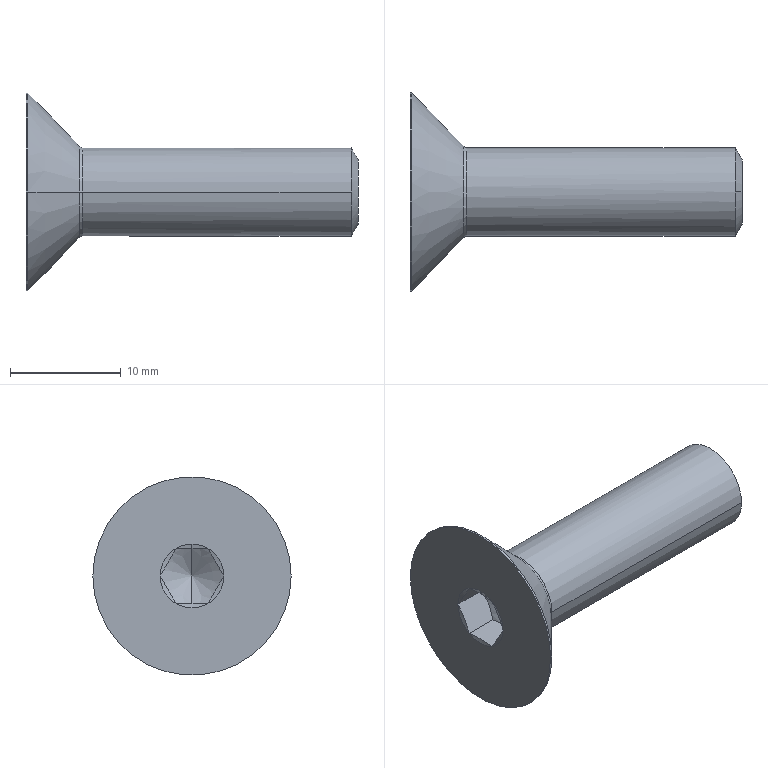Part | SolidWorks | features BaseBody 1 | 1 solid | 27 faces | box 30 x 17.92 x 17.92 mm | volume 1877 mm3 | cone 13 | plane 8 | cylinder 4 | spline 2 | commonest cylinder face diameters 8 x2 17.92 x2
STEP:
#1=CARTESIAN_POINT('',(-25.158,-4.122,0.));
#2=VERTEX_POINT('',#1);
#3=CARTESIAN_POINT('',(-25.158,4.122,0.));
#4=VERTEX_POINT('',#3);
#5=CARTESIAN_POINT('',(-25.158,0.,0.));
#6=DIRECTION('',(-1.,0.,0.));
#7=DIRECTION('',(0.,1.,0.));
#8=AXIS2_PLACEMENT_3D('',#5,#6,#7);
#9=CIRCLE('',#8,4.122);
#10=EDGE_CURVE('',#2,#4,#9,.T.);
#11=ORIENTED_EDGE('',*,*,#10,.F.);
#12=CARTESIAN_POINT('',(-24.87,-4.,0.));
#13=VERTEX_POINT('',#12);
#14=CARTESIAN_POINT('',(-24.87,-4.4,0.));
#15=DIRECTION('',(0.,0.,-1.));
#16=DIRECTION('',(0.,-1.,0.));
#17=AXIS2_PLACEMENT_3D('',#14,#15,#16);
#18=CIRCLE('',#17,0.4);
#19=EDGE_CURVE('',#2,#13,#18,.T.);
#20=ORIENTED_EDGE('',*,*,#19,.T.);
#21=CARTESIAN_POINT('',(-24.87,4.,0.));
#22=VERTEX_POINT('',#21);
#23=CARTESIAN_POINT('',(-24.87,0.,0.));
#24=DIRECTION('',(1.,0.,0.));
#25=DIRECTION('',(0.,1.,0.));
#26=AXIS2_PLACEMENT_3D('',#23,#24,#25);
#27=CIRCLE('',#26,4.);
#28=EDGE_CURVE('',#22,#13,#27,.T.);
#29=ORIENTED_EDGE('',*,*,#28,.F.);
#30=CARTESIAN_POINT('',(-24.87,4.4,0.));
#31=DIRECTION('',(0.,0.,1.));
#32=DIRECTION('',(0.,1.,0.));
#33=AXIS2_PLACEMENT_3D('',#30,#31,#32);
#34=CIRCLE('',#33,0.4);
#35=EDGE_CURVE('',#4,#22,#34,.T.);
#36=ORIENTED_EDGE('',*,*,#35,.F.);
#37=EDGE_LOOP('',(#11,#20,#29,#36));
#38=FACE_OUTER_BOUND('',#37,.T.);
#39=CARTESIAN_POINT('',(-25.158,4.122,0.));
#40=CARTESIAN_POINT('',(-25.158,4.122,8.244));
#41=CARTESIAN_POINT('',(-25.158,-4.122,8.244));
#42=CARTESIAN_POINT('',(-25.158,-4.122,0.));
#43=CARTESIAN_POINT('',(-25.082,4.043,0.));
#44=CARTESIAN_POINT('',(-25.082,4.043,8.086));
#45=CARTESIAN_POINT('',(-25.082,-4.043,8.086));
#46=CARTESIAN_POINT('',(-25.082,-4.043,0.));
#47=CARTESIAN_POINT('',(-24.98,4.,0.));
#48=CARTESIAN_POINT('',(-24.98,4.,8.));
#49=CARTESIAN_POINT('',(-24.98,-4.,8.));
#50=CARTESIAN_POINT('',(-24.98,-4.,0.));
#51=CARTESIAN_POINT('',(-24.87,4.,0.));
#52=CARTESIAN_POINT('',(-24.87,4.,8.));
#53=CARTESIAN_POINT('',(-24.87,-4.,8.));
#54=CARTESIAN_POINT('',(-24.87,-4.,0.));
#55=(BOUNDED_SURFACE()B_SPLINE_SURFACE(3,3,((#39,#40,#41,#42),(#43,#44,#45,#46),(#47,#48,#49,#50),(#51,#52,#53,#54)),.UNSPECIFIED.,.F.,.F.,.T.)B_SPLINE_SURFACE_WITH_KNOTS((4,4),(4,4),(0.,1.),(0.,1.),.UNSPECIFIED.)GEOMETRIC_REPRESENTATION_ITEM()RATIONAL_B_SPLINE_SURFACE(((1.,0.3333,0.3333,1.),(0.947,0.3157,0.3157,0.947),(0.947,0.3157,0.3157,0.947),(1.,0.3333,0.3333,1.)))REPRESENTATION_ITEM('')SURFACE());
#56=ADVANCED_FACE('',(#38),#55,.F.);
#57=ORIENTED_EDGE('',*,*,#28,.T.);
#58=CARTESIAN_POINT('',(-0.625,-4.,0.));
#59=VERTEX_POINT('',#58);
#60=CARTESIAN_POINT('',(0.,-4.,0.));
#61=DIRECTION('',(1.,0.,0.));
#62=VECTOR('',#61,1000.);
#63=LINE('',#60,#62);
#64=EDGE_CURVE('',#13,#59,#63,.T.);
#65=ORIENTED_EDGE('',*,*,#64,.T.);
#66=CARTESIAN_POINT('',(-0.625,0.,4.));
#67=VERTEX_POINT('',#66);
#68=CARTESIAN_POINT('',(-0.625,0.,0.));
#69=DIRECTION('',(-1.,0.,0.));
#70=DIRECTION('',(0.,1.,0.));
#71=AXIS2_PLACEMENT_3D('',#68,#69,#70);
#72=CIRCLE('',#71,4.);
#73=EDGE_CURVE('',#59,#67,#72,.T.);
#74=ORIENTED_EDGE('',*,*,#73,.T.);
#75=CARTESIAN_POINT('',(-0.625,4.,0.));
#76=VERTEX_POINT('',#75);
#77=CARTESIAN_POINT('',(-0.625,0.,0.));
#78=DIRECTION('',(-1.,0.,0.));
#79=DIRECTION('',(0.,1.,0.));
#80=AXIS2_PLACEMENT_3D('',#77,#78,#79);
#81=CIRCLE('',#80,4.);
#82=EDGE_CURVE('',#67,#76,#81,.T.);
#83=ORIENTED_EDGE('',*,*,#82,.T.);
#84=CARTESIAN_POINT('',(0.,4.,0.));
#85=DIRECTION('',(1.,0.,0.));
#86=VECTOR('',#85,1000.);
#87=LINE('',#84,#86);
#88=EDGE_CURVE('',#22,#76,#87,.T.);
#89=ORIENTED_EDGE('',*,*,#88,.F.);
#90=EDGE_LOOP('',(#57,#65,#74,#83,#89));
#91=FACE_OUTER_BOUND('',#90,.T.);
#92=CARTESIAN_POINT('',(0.,0.,0.));
#93=DIRECTION('',(1.,0.,0.));
#94=DIRECTION('',(0.,1.,0.));
#95=AXIS2_PLACEMENT_3D('',#92,#93,#94);
#96=CYLINDRICAL_SURFACE('',#95,4.);
#97=ADVANCED_FACE('',(#91),#96,.T.);
#98=CARTESIAN_POINT('',(0.,0.,2.917));
#99=VERTEX_POINT('',#98);
#100=CARTESIAN_POINT('',(0.,0.,-2.917));
#101=VERTEX_POINT('',#100);
#102=CARTESIAN_POINT('',(0.,0.,0.));
#103=DIRECTION('',(-1.,0.,0.));
#104=DIRECTION('',(0.,0.,1.));
#105=AXIS2_PLACEMENT_3D('',#102,#103,#104);
#106=CIRCLE('',#105,2.917);
#107=EDGE_CURVE('',#99,#101,#106,.T.);
#108=ORIENTED_EDGE('',*,*,#107,.T.);
#109=CARTESIAN_POINT('',(-0.625,0.,-4.));
#110=VERTEX_POINT('',#109);
#111=CARTESIAN_POINT('',(-0.625,0.,-4.));
#112=DIRECTION('',(-0.5,0.,-0.866));
#113=VECTOR('',#112,1000.);
#114=LINE('',#111,#113);
#115=EDGE_CURVE('',#101,#110,#114,.T.);
#116=ORIENTED_EDGE('',*,*,#115,.T.);
#117=CARTESIAN_POINT('',(-0.625,0.,0.));
#118=DIRECTION('',(-1.,0.,0.));
#119=DIRECTION('',(0.,1.,0.));
#120=AXIS2_PLACEMENT_3D('',#117,#118,#119);
#121=CIRCLE('',#120,4.);
#122=EDGE_CURVE('',#76,#110,#121,.T.);
#123=ORIENTED_EDGE('',*,*,#122,.F.);
#124=ORIENTED_EDGE('',*,*,#82,.F.);
#125=CARTESIAN_POINT('',(-0.625,0.,4.));
#126=DIRECTION('',(-0.5,0.,0.866));
#127=VECTOR('',#126,1000.);
#128=LINE('',#125,#127);
#129=EDGE_CURVE('',#99,#67,#128,.T.);
#130=ORIENTED_EDGE('',*,*,#129,.F.);
#131=EDGE_LOOP('',(#108,#116,#123,#124,#130));
#132=FACE_OUTER_BOUND('',#131,.T.);
#133=CARTESIAN_POINT('',(-0.625,0.,0.));
#134=DIRECTION('',(-1.,0.,0.));
#135=DIRECTION('',(0.,0.,1.));
#136=AXIS2_PLACEMENT_3D('',#133,#134,#135);
#137=CONICAL_SURFACE('',#136,4.,1.047);
#138=ADVANCED_FACE('',(#132),#137,.T.);
#139=ORIENTED_EDGE('',*,*,#10,.T.);
#140=CARTESIAN_POINT('',(-29.83,8.96,0.));
#141=VERTEX_POINT('',#140);
#142=CARTESIAN_POINT('',(-29.83,8.96,0.));
#143=DIRECTION('',(-0.6947,0.7193,0.));
#144=VECTOR('',#143,1000.);
#145=LINE('',#142,#144);
#146=EDGE_CURVE('',#4,#141,#145,.T.);
#147=ORIENTED_EDGE('',*,*,#146,.T.);
#148=CARTESIAN_POINT('',(-29.83,-8.96,0.));
#149=VERTEX_POINT('',#148);
#150=CARTESIAN_POINT('',(-29.83,0.,0.));
#151=DIRECTION('',(1.,0.,0.));
#152=DIRECTION('',(0.,-1.,0.));
#153=AXIS2_PLACEMENT_3D('',#150,#151,#152);
#154=CIRCLE('',#153,8.96);
#155=EDGE_CURVE('',#141,#149,#154,.T.);
#156=ORIENTED_EDGE('',*,*,#155,.T.);
#157=CARTESIAN_POINT('',(-29.83,-8.96,0.));
#158=DIRECTION('',(-0.6947,-0.7193,0.));
#159=VECTOR('',#158,1000.);
#160=LINE('',#157,#159);
#161=EDGE_CURVE('',#2,#149,#160,.T.);
#162=ORIENTED_EDGE('',*,*,#161,.F.);
#163=EDGE_LOOP('',(#139,#147,#156,#162));
#164=FACE_OUTER_BOUND('',#163,.T.);
#165=CARTESIAN_POINT('',(-29.83,0.,0.));
#166=DIRECTION('',(-1.,0.,0.));
#167=DIRECTION('',(0.,-1.,0.));
#168=AXIS2_PLACEMENT_3D('',#165,#166,#167);
#169=CONICAL_SURFACE('',#168,8.96,0.8029);
#170=ADVANCED_FACE('',(#164),#169,.T.);
#171=CARTESIAN_POINT('',(-30.,8.96,0.));
#172=VERTEX_POINT('',#171);
#173=CARTESIAN_POINT('',(-30.,-8.96,0.));
#174=VERTEX_POINT('',#173);
#175=CARTESIAN_POINT('',(-30.,0.,0.));
#176=DIRECTION('',(1.,0.,0.));
#177=DIRECTION('',(0.,1.,0.));
#178=AXIS2_PLACEMENT_3D('',#175,#176,#177);
#179=CIRCLE('',#178,8.96);
#180=EDGE_CURVE('',#172,#174,#179,.T.);
#181=ORIENTED_EDGE('',*,*,#180,.T.);
#182=CARTESIAN_POINT('',(0.,-8.96,0.));
#183=DIRECTION('',(1.,0.,0.));
#184=VECTOR('',#183,1000.);
#185=LINE('',#182,#184);
#186=EDGE_CURVE('',#174,#149,#185,.T.);
#187=ORIENTED_EDGE('',*,*,#186,.T.);
#188=ORIENTED_EDGE('',*,*,#155,.F.);
#189=CARTESIAN_POINT('',(0.,8.96,0.));
#190=DIRECTION('',(1.,0.,0.));
#191=VECTOR('',#190,1000.);
#192=LINE('',#189,#191);
#193=EDGE_CURVE('',#172,#141,#192,.T.);
#194=ORIENTED_EDGE('',*,*,#193,.F.);
#195=EDGE_LOOP('',(#181,#187,#188,#194));
#196=FACE_OUTER_BOUND('',#195,.T.);
#197=CARTESIAN_POINT('',(0.,0.,0.));
#198=DIRECTION('',(1.,0.,0.));
#199=DIRECTION('',(0.,1.,0.));
#200=AXIS2_PLACEMENT_3D('',#197,#198,#199);
#201=CYLINDRICAL_SURFACE('',#200,8.96);
#202=ADVANCED_FACE('',(#196),#201,.T.);
#203=CARTESIAN_POINT('',(-30.,1.443,2.5));
#204=VERTEX_POINT('',#203);
#205=CARTESIAN_POINT('',(-29.894,0.,2.5));
#206=VERTEX_POINT('',#205);
#207=CARTESIAN_POINT('',(-30.,1.443,2.5));
#208=CARTESIAN_POINT('',(-29.934,0.9645,2.5));
#209=CARTESIAN_POINT('',(-29.894,0.4837,2.5));
#210=CARTESIAN_POINT('',(-29.894,0.,2.5));
#211=B_SPLINE_CURVE_WITH_KNOTS('',3,(#207,#208,#209,#210),.UNSPECIFIED.,.F.,.F.,(4,4),(0.,0.001447),.UNSPECIFIED.);
#212=EDGE_CURVE('',#204,#206,#211,.T.);
#213=ORIENTED_EDGE('',*,*,#212,.T.);
#214=CARTESIAN_POINT('',(-30.,0.,2.887));
#215=VERTEX_POINT('',#214);
#216=CARTESIAN_POINT('',(-30.,0.,2.887));
#217=DIRECTION('',(-0.2646,0.,0.9644));
#218=VECTOR('',#217,1000.);
#219=LINE('',#216,#218);
#220=EDGE_CURVE('',#206,#215,#219,.T.);
#221=ORIENTED_EDGE('',*,*,#220,.T.);
#222=CARTESIAN_POINT('',(-30.,0.,0.));
#223=DIRECTION('',(1.,0.,0.));
#224=DIRECTION('',(0.,0.,1.));
#225=AXIS2_PLACEMENT_3D('',#222,#223,#224);
#226=CIRCLE('',#225,2.887);
#227=EDGE_CURVE('',#204,#215,#226,.T.);
#228=ORIENTED_EDGE('',*,*,#227,.F.);
#229=EDGE_LOOP('',(#213,#221,#228));
#230=FACE_OUTER_BOUND('',#229,.T.);
#231=CARTESIAN_POINT('',(-30.,0.,0.));
#232=DIRECTION('',(-1.,0.,0.));
#233=DIRECTION('',(0.,0.,1.));
#234=AXIS2_PLACEMENT_3D('',#231,#232,#233);
#235=CONICAL_SURFACE('',#234,2.887,1.303);
#236=ADVANCED_FACE('',(#230),#235,.F.);
#237=CARTESIAN_POINT('',(-25.333,0.,0.));
#238=VERTEX_POINT('',#237);
#239=CARTESIAN_POINT('',(-26.777,0.,2.5));
#240=VERTEX_POINT('',#239);
#241=CARTESIAN_POINT('',(-27.01,0.,2.904));
#242=DIRECTION('',(-0.5,0.,0.866));
#243=VECTOR('',#242,1000.);
#244=LINE('',#241,#243);
#245=EDGE_CURVE('',#238,#240,#244,.T.);
#246=ORIENTED_EDGE('',*,*,#245,.F.);
#247=CARTESIAN_POINT('',(-26.777,0.,-2.5));
#248=VERTEX_POINT('',#247);
#249=CARTESIAN_POINT('',(-27.01,0.,-2.904));
#250=DIRECTION('',(-0.5,0.,-0.866));
#251=VECTOR('',#250,1000.);
#252=LINE('',#249,#251);
#253=EDGE_CURVE('',#238,#248,#252,.T.);
#254=ORIENTED_EDGE('',*,*,#253,.T.);
#255=CARTESIAN_POINT('',(-27.,-1.443,-2.5));
#256=VERTEX_POINT('',#255);
#257=CARTESIAN_POINT('',(-26.777,0.,-2.5));
#258=CARTESIAN_POINT('',(-26.777,-0.4926,-2.5));
#259=CARTESIAN_POINT('',(-26.864,-0.9718,-2.5));
#260=CARTESIAN_POINT('',(-27.,-1.443,-2.5));
#261=B_SPLINE_CURVE_WITH_KNOTS('',3,(#257,#258,#259,#260),.UNSPECIFIED.,.F.,.F.,(4,4),(0.001461,0.002921),.UNSPECIFIED.);
#262=EDGE_CURVE('',#248,#256,#261,.T.);
#263=ORIENTED_EDGE('',*,*,#262,.T.);
#264=CARTESIAN_POINT('',(-27.,-2.887,0.));
#265=VERTEX_POINT('',#264);
#266=CARTESIAN_POINT('',(-27.,-1.443,-2.5));
#267=CARTESIAN_POINT('',(-26.864,-1.679,-2.092));
#268=CARTESIAN_POINT('',(-26.777,-1.918,-1.677));
#269=CARTESIAN_POINT('',(-26.777,-2.286,-1.04));
#270=CARTESIAN_POINT('',(-26.798,-2.409,-0.8275));
#271=CARTESIAN_POINT('',(-26.876,-2.65,-0.4104));
#272=CARTESIAN_POINT('',(-26.932,-2.769,-0.2044));
#273=CARTESIAN_POINT('',(-27.,-2.887,0.));
#274=B_SPLINE_CURVE_WITH_KNOTS('',3,(#266,#267,#268,#269,#270,#271,#272,#273),.UNSPECIFIED.,.F.,.F.,(4,2,2,4),(0.,0.001458,0.002187,0.002915),.UNSPECIFIED.);
#275=EDGE_CURVE('',#256,#265,#274,.T.);
#276=ORIENTED_EDGE('',*,*,#275,.T.);
#277=CARTESIAN_POINT('',(-27.,-1.443,2.5));
#278=VERTEX_POINT('',#277);
#279=CARTESIAN_POINT('',(-27.,-2.887,0.));
#280=CARTESIAN_POINT('',(-26.864,-2.651,0.4082));
#281=CARTESIAN_POINT('',(-26.777,-2.412,0.8225));
#282=CARTESIAN_POINT('',(-26.777,-2.044,1.46));
#283=CARTESIAN_POINT('',(-26.798,-1.921,1.672));
#284=CARTESIAN_POINT('',(-26.876,-1.68,2.09));
#285=CARTESIAN_POINT('',(-26.932,-1.561,2.296));
#286=CARTESIAN_POINT('',(-27.,-1.443,2.5));
#287=B_SPLINE_CURVE_WITH_KNOTS('',3,(#279,#280,#281,#282,#283,#284,#285,#286),.UNSPECIFIED.,.F.,.F.,(4,2,2,4),(0.,0.001458,0.002187,0.002915),.UNSPECIFIED.);
#288=EDGE_CURVE('',#265,#278,#287,.T.);
#289=ORIENTED_EDGE('',*,*,#288,.T.);
#290=CARTESIAN_POINT('',(-26.777,0.,2.5));
#291=CARTESIAN_POINT('',(-26.777,-0.4926,2.5));
#292=CARTESIAN_POINT('',(-26.864,-0.9718,2.5));
#293=CARTESIAN_POINT('',(-27.,-1.443,2.5));
#294=B_SPLINE_CURVE_WITH_KNOTS('',3,(#290,#291,#292,#293),.UNSPECIFIED.,.F.,.F.,(4,4),(0.001461,0.002921),.UNSPECIFIED.);
#295=EDGE_CURVE('',#240,#278,#294,.T.);
#296=ORIENTED_EDGE('',*,*,#295,.F.);
#297=EDGE_LOOP('',(#246,#254,#263,#276,#289,#296));
#298=FACE_OUTER_BOUND('',#297,.T.);
#299=CARTESIAN_POINT('',(-27.01,0.,0.));
#300=DIRECTION('',(-1.,0.,0.));
#301=DIRECTION('',(0.,0.,1.));
#302=AXIS2_PLACEMENT_3D('',#299,#300,#301);
#303=CONICAL_SURFACE('',#302,2.904,1.047);
#304=ADVANCED_FACE('',(#298),#303,.F.);
#305=ORIENTED_EDGE('',*,*,#64,.F.);
#306=CARTESIAN_POINT('',(-24.87,0.,0.));
#307=DIRECTION('',(1.,0.,0.));
#308=DIRECTION('',(0.,1.,0.));
#309=AXIS2_PLACEMENT_3D('',#306,#307,#308);
#310=CIRCLE('',#309,4.);
#311=EDGE_CURVE('',#13,#22,#310,.T.);
#312=ORIENTED_EDGE('',*,*,#311,.T.);
#313=ORIENTED_EDGE('',*,*,#88,.T.);
#314=ORIENTED_EDGE('',*,*,#122,.T.);
#315=CARTESIAN_POINT('',(-0.625,0.,0.));
#316=DIRECTION('',(-1.,0.,0.));
#317=DIRECTION('',(0.,1.,0.));
#318=AXIS2_PLACEMENT_3D('',#315,#316,#317);
#319=CIRCLE('',#318,4.);
#320=EDGE_CURVE('',#110,#59,#319,.T.);
#321=ORIENTED_EDGE('',*,*,#320,.T.);
#322=EDGE_LOOP('',(#305,#312,#313,#314,#321));
#323=FACE_OUTER_BOUND('',#322,.T.);
#324=CARTESIAN_POINT('',(0.,0.,0.));
#325=DIRECTION('',(1.,0.,0.));
#326=DIRECTION('',(0.,1.,0.));
#327=AXIS2_PLACEMENT_3D('',#324,#325,#326);
#328=CYLINDRICAL_SURFACE('',#327,4.);
#329=ADVANCED_FACE('',(#323),#328,.T.);
#330=ORIENTED_EDGE('',*,*,#115,.F.);
#331=CARTESIAN_POINT('',(0.,0.,0.));
#332=DIRECTION('',(-1.,0.,0.));
#333=DIRECTION('',(0.,0.,1.));
#334=AXIS2_PLACEMENT_3D('',#331,#332,#333);
#335=CIRCLE('',#334,2.917);
#336=EDGE_CURVE('',#101,#99,#335,.T.);
#337=ORIENTED_EDGE('',*,*,#336,.T.);
#338=ORIENTED_EDGE('',*,*,#129,.T.);
#339=ORIENTED_EDGE('',*,*,#73,.F.);
#340=ORIENTED_EDGE('',*,*,#320,.F.);
#341=EDGE_LOOP('',(#330,#337,#338,#339,#340));
#342=FACE_OUTER_BOUND('',#341,.T.);
#343=CARTESIAN_POINT('',(-0.625,0.,0.));
#344=DIRECTION('',(-1.,0.,0.));
#345=DIRECTION('',(0.,0.,1.));
#346=AXIS2_PLACEMENT_3D('',#343,#344,#345);
#347=CONICAL_SURFACE('',#346,4.,1.047);
#348=ADVANCED_FACE('',(#342),#347,.T.);
#349=ORIENTED_EDGE('',*,*,#19,.F.);
#350=CARTESIAN_POINT('',(-25.158,0.,0.));
#351=DIRECTION('',(-1.,0.,0.));
#352=DIRECTION('',(0.,1.,0.));
#353=AXIS2_PLACEMENT_3D('',#350,#351,#352);
#354=CIRCLE('',#353,4.122);
#355=EDGE_CURVE('',#4,#2,#354,.T.);
#356=ORIENTED_EDGE('',*,*,#355,.F.);
#357=ORIENTED_EDGE('',*,*,#35,.T.);
#358=ORIENTED_EDGE('',*,*,#311,.F.);
#359=EDGE_LOOP('',(#349,#356,#357,#358));
#360=FACE_OUTER_BOUND('',#359,.T.);
#361=CARTESIAN_POINT('',(-25.158,-4.122,0.));
#362=CARTESIAN_POINT('',(-25.158,-4.122,-8.244));
#363=CARTESIAN_POINT('',(-25.158,4.122,-8.244));
#364=CARTESIAN_POINT('',(-25.158,4.122,0.));
#365=CARTESIAN_POINT('',(-25.082,-4.043,0.));
#366=CARTESIAN_POINT('',(-25.082,-4.043,-8.086));
#367=CARTESIAN_POINT('',(-25.082,4.043,-8.086));
#368=CARTESIAN_POINT('',(-25.082,4.043,0.));
#369=CARTESIAN_POINT('',(-24.98,-4.,0.));
#370=CARTESIAN_POINT('',(-24.98,-4.,-8.));
#371=CARTESIAN_POINT('',(-24.98,4.,-8.));
#372=CARTESIAN_POINT('',(-24.98,4.,0.));
#373=CARTESIAN_POINT('',(-24.87,-4.,0.));
#374=CARTESIAN_POINT('',(-24.87,-4.,-8.));
#375=CARTESIAN_POINT('',(-24.87,4.,-8.));
#376=CARTESIAN_POINT('',(-24.87,4.,0.));
#377=(BOUNDED_SURFACE()B_SPLINE_SURFACE(3,3,((#361,#362,#363,#364),(#365,#366,#367,#368),(#369,#370,#371,#372),(#373,#374,#375,#376)),.UNSPECIFIED.,.F.,.F.,.F.)B_SPLINE_SURFACE_WITH_KNOTS((4,4),(4,4),(0.,1.),(0.,1.),.UNSPECIFIED.)GEOMETRIC_REPRESENTATION_ITEM()RATIONAL_B_SPLINE_SURFACE(((1.,0.3333,0.3333,1.),(0.947,0.3157,0.3157,0.947),(0.947,0.3157,0.3157,0.947),(1.,0.3333,0.3333,1.)))REPRESENTATION_ITEM('')SURFACE());
#378=ADVANCED_FACE('',(#360),#377,.F.);
#379=ORIENTED_EDGE('',*,*,#107,.F.);
#380=ORIENTED_EDGE('',*,*,#336,.F.);
#381=EDGE_LOOP('',(#379,#380));
#382=FACE_OUTER_BOUND('',#381,.T.);
#383=CARTESIAN_POINT('',(0.,0.,0.));
#384=DIRECTION('',(1.,0.,0.));
#385=DIRECTION('',(0.,1.,0.));
#386=AXIS2_PLACEMENT_3D('',#383,#384,#385);
#387=PLANE('',#386);
#388=ADVANCED_FACE('',(#382),#387,.T.);
#389=ORIENTED_EDGE('',*,*,#146,.F.);
#390=ORIENTED_EDGE('',*,*,#355,.T.);
#391=ORIENTED_EDGE('',*,*,#161,.T.);
#392=CARTESIAN_POINT('',(-29.83,0.,0.));
#393=DIRECTION('',(1.,0.,0.));
#394=DIRECTION('',(0.,-1.,0.));
#395=AXIS2_PLACEMENT_3D('',#392,#393,#394);
#396=CIRCLE('',#395,8.96);
#397=EDGE_CURVE('',#149,#141,#396,.T.);
#398=ORIENTED_EDGE('',*,*,#397,.T.);
#399=EDGE_LOOP('',(#389,#390,#391,#398));
#400=FACE_OUTER_BOUND('',#399,.T.);
#401=CARTESIAN_POINT('',(-29.83,0.,0.));
#402=DIRECTION('',(-1.,0.,0.));
#403=DIRECTION('',(0.,-1.,0.));
#404=AXIS2_PLACEMENT_3D('',#401,#402,#403);
#405=CONICAL_SURFACE('',#404,8.96,0.8029);
#406=ADVANCED_FACE('',(#400),#405,.T.);
#407=ORIENTED_EDGE('',*,*,#186,.F.);
#408=CARTESIAN_POINT('',(-30.,0.,0.));
#409=DIRECTION('',(1.,0.,0.));
#410=DIRECTION('',(0.,1.,0.));
#411=AXIS2_PLACEMENT_3D('',#408,#409,#410);
#412=CIRCLE('',#411,8.96);
#413=EDGE_CURVE('',#174,#172,#412,.T.);
#414=ORIENTED_EDGE('',*,*,#413,.T.);
#415=ORIENTED_EDGE('',*,*,#193,.T.);
#416=ORIENTED_EDGE('',*,*,#397,.F.);
#417=EDGE_LOOP('',(#407,#414,#415,#416));
#418=FACE_OUTER_BOUND('',#417,.T.);
#419=CARTESIAN_POINT('',(0.,0.,0.));
#420=DIRECTION('',(1.,0.,0.));
#421=DIRECTION('',(0.,1.,0.));
#422=AXIS2_PLACEMENT_3D('',#419,#420,#421);
#423=CYLINDRICAL_SURFACE('',#422,8.96);
#424=ADVANCED_FACE('',(#418),#423,.T.);
#425=CARTESIAN_POINT('',(-30.,2.887,0.));
#426=VERTEX_POINT('',#425);
#427=CARTESIAN_POINT('',(-30.,0.,0.));
#428=DIRECTION('',(1.,0.,0.));
#429=DIRECTION('',(0.,0.,1.));
#430=AXIS2_PLACEMENT_3D('',#427,#428,#429);
#431=CIRCLE('',#430,2.887);
#432=EDGE_CURVE('',#426,#204,#431,.T.);
#433=ORIENTED_EDGE('',*,*,#432,.T.);
#434=ORIENTED_EDGE('',*,*,#227,.T.);
#435=CARTESIAN_POINT('',(-30.,-1.443,2.5));
#436=VERTEX_POINT('',#435);
#437=CARTESIAN_POINT('',(-30.,0.,0.));
#438=DIRECTION('',(1.,0.,0.));
#439=DIRECTION('',(0.,0.,1.));
#440=AXIS2_PLACEMENT_3D('',#437,#438,#439);
#441=CIRCLE('',#440,2.887);
#442=EDGE_CURVE('',#215,#436,#441,.T.);
#443=ORIENTED_EDGE('',*,*,#442,.T.);
#444=CARTESIAN_POINT('',(-30.,-2.887,0.));
#445=VERTEX_POINT('',#444);
#446=CARTESIAN_POINT('',(-30.,0.,0.));
#447=DIRECTION('',(1.,0.,0.));
#448=DIRECTION('',(0.,0.,1.));
#449=AXIS2_PLACEMENT_3D('',#446,#447,#448);
#450=CIRCLE('',#449,2.887);
#451=EDGE_CURVE('',#436,#445,#450,.T.);
#452=ORIENTED_EDGE('',*,*,#451,.T.);
#453=CARTESIAN_POINT('',(-30.,-1.443,-2.5));
#454=VERTEX_POINT('',#453);
#455=CARTESIAN_POINT('',(-30.,0.,0.));
#456=DIRECTION('',(1.,0.,0.));
#457=DIRECTION('',(0.,0.,1.));
#458=AXIS2_PLACEMENT_3D('',#455,#456,#457);
#459=CIRCLE('',#458,2.887);
#460=EDGE_CURVE('',#445,#454,#459,.T.);
#461=ORIENTED_EDGE('',*,*,#460,.T.);
#462=CARTESIAN_POINT('',(-30.,1.443,-2.5));
#463=VERTEX_POINT('',#462);
#464=CARTESIAN_POINT('',(-30.,0.,0.));
#465=DIRECTION('',(1.,0.,0.));
#466=DIRECTION('',(0.,0.,1.));
#467=AXIS2_PLACEMENT_3D('',#464,#465,#466);
#468=CIRCLE('',#467,2.887);
#469=EDGE_CURVE('',#454,#463,#468,.T.);
#470=ORIENTED_EDGE('',*,*,#469,.T.);
#471=CARTESIAN_POINT('',(-30.,0.,0.));
#472=DIRECTION('',(1.,0.,0.));
#473=DIRECTION('',(0.,0.,1.));
#474=AXIS2_PLACEMENT_3D('',#471,#472,#473);
#475=CIRCLE('',#474,2.887);
#476=EDGE_CURVE('',#463,#426,#475,.T.);
#477=ORIENTED_EDGE('',*,*,#476,.T.);
#478=EDGE_LOOP('',(#433,#434,#443,#452,#461,#470,#477));
#479=FACE_BOUND('',#478,.T.);
#480=ORIENTED_EDGE('',*,*,#180,.F.);
#481=ORIENTED_EDGE('',*,*,#413,.F.);
#482=EDGE_LOOP('',(#480,#481));
#483=FACE_OUTER_BOUND('',#482,.T.);
#484=CARTESIAN_POINT('',(-30.,8.96,0.));
#485=DIRECTION('',(-1.,0.,0.));
#486=DIRECTION('',(0.,-1.,0.));
#487=AXIS2_PLACEMENT_3D('',#484,#485,#486);
#488=PLANE('',#487);
#489=ADVANCED_FACE('',(#479,#483),#488,.T.);
#490=ORIENTED_EDGE('',*,*,#220,.F.);
#491=CARTESIAN_POINT('',(-29.894,0.,2.5));
#492=CARTESIAN_POINT('',(-29.894,-0.4837,2.5));
#493=CARTESIAN_POINT('',(-29.934,-0.9645,2.5));
#494=CARTESIAN_POINT('',(-30.,-1.443,2.5));
#495=B_SPLINE_CURVE_WITH_KNOTS('',3,(#491,#492,#493,#494),.UNSPECIFIED.,.F.,.F.,(4,4),(0.001447,0.002895),.UNSPECIFIED.);
#496=EDGE_CURVE('',#206,#436,#495,.T.);
#497=ORIENTED_EDGE('',*,*,#496,.T.);
#498=ORIENTED_EDGE('',*,*,#442,.F.);
#499=EDGE_LOOP('',(#490,#497,#498));
#500=FACE_OUTER_BOUND('',#499,.T.);
#501=CARTESIAN_POINT('',(-30.,0.,0.));
#502=DIRECTION('',(-1.,0.,0.));
#503=DIRECTION('',(0.,0.,1.));
#504=AXIS2_PLACEMENT_3D('',#501,#502,#503);
#505=CONICAL_SURFACE('',#504,2.887,1.303);
#506=ADVANCED_FACE('',(#500),#505,.F.);
#507=ORIENTED_EDGE('',*,*,#432,.F.);
#508=CARTESIAN_POINT('',(-30.,1.443,2.5));
#509=CARTESIAN_POINT('',(-29.934,1.684,2.083));
#510=CARTESIAN_POINT('',(-29.854,2.165,1.25));
#511=CARTESIAN_POINT('',(-29.934,2.646,0.4167));
#512=CARTESIAN_POINT('',(-30.,2.887,0.));
#513=B_SPLINE_CURVE_WITH_KNOTS('',3,(#508,#509,#510,#511,#512),.UNSPECIFIED.,.F.,.F.,(4,1,4),(0.,0.001443,0.002887),.UNSPECIFIED.);
#514=EDGE_CURVE('',#204,#426,#513,.T.);
#515=ORIENTED_EDGE('',*,*,#514,.F.);
#516=EDGE_LOOP('',(#507,#515));
#517=FACE_OUTER_BOUND('',#516,.T.);
#518=CARTESIAN_POINT('',(-30.,0.,0.));
#519=DIRECTION('',(-1.,0.,0.));
#520=DIRECTION('',(0.,0.,1.));
#521=AXIS2_PLACEMENT_3D('',#518,#519,#520);
#522=CONICAL_SURFACE('',#521,2.887,1.303);
#523=ADVANCED_FACE('',(#517),#522,.F.);
#524=ORIENTED_EDGE('',*,*,#476,.F.);
#525=CARTESIAN_POINT('',(-30.,2.887,0.));
#526=CARTESIAN_POINT('',(-29.934,2.646,-0.4167));
#527=CARTESIAN_POINT('',(-29.854,2.165,-1.25));
#528=CARTESIAN_POINT('',(-29.934,1.684,-2.083));
#529=CARTESIAN_POINT('',(-30.,1.443,-2.5));
#530=B_SPLINE_CURVE_WITH_KNOTS('',3,(#525,#526,#527,#528,#529),.UNSPECIFIED.,.F.,.F.,(4,1,4),(0.,0.001443,0.002887),.UNSPECIFIED.);
#531=EDGE_CURVE('',#426,#463,#530,.T.);
#532=ORIENTED_EDGE('',*,*,#531,.F.);
#533=EDGE_LOOP('',(#524,#532));
#534=FACE_OUTER_BOUND('',#533,.T.);
#535=CARTESIAN_POINT('',(-30.,0.,0.));
#536=DIRECTION('',(-1.,0.,0.));
#537=DIRECTION('',(0.,0.,1.));
#538=AXIS2_PLACEMENT_3D('',#535,#536,#537);
#539=CONICAL_SURFACE('',#538,2.887,1.303);
#540=ADVANCED_FACE('',(#534),#539,.F.);
#541=ORIENTED_EDGE('',*,*,#469,.F.);
#542=CARTESIAN_POINT('',(-30.,1.443,-2.5));
#543=CARTESIAN_POINT('',(-29.934,0.9623,-2.5));
#544=CARTESIAN_POINT('',(-29.854,0.,-2.5));
#545=CARTESIAN_POINT('',(-29.934,-0.9623,-2.5));
#546=CARTESIAN_POINT('',(-30.,-1.443,-2.5));
#547=B_SPLINE_CURVE_WITH_KNOTS('',3,(#542,#543,#544,#545,#546),.UNSPECIFIED.,.F.,.F.,(4,1,4),(0.,0.001443,0.002887),.UNSPECIFIED.);
#548=EDGE_CURVE('',#463,#454,#547,.T.);
#549=ORIENTED_EDGE('',*,*,#548,.F.);
#550=EDGE_LOOP('',(#541,#549));
#551=FACE_OUTER_BOUND('',#550,.T.);
#552=CARTESIAN_POINT('',(-30.,0.,0.));
#553=DIRECTION('',(-1.,0.,0.));
#554=DIRECTION('',(0.,0.,1.));
#555=AXIS2_PLACEMENT_3D('',#552,#553,#554);
#556=CONICAL_SURFACE('',#555,2.887,1.303);
#557=ADVANCED_FACE('',(#551),#556,.F.);
#558=ORIENTED_EDGE('',*,*,#460,.F.);
#559=CARTESIAN_POINT('',(-30.,-1.443,-2.5));
#560=CARTESIAN_POINT('',(-29.934,-1.684,-2.083));
#561=CARTESIAN_POINT('',(-29.854,-2.165,-1.25));
#562=CARTESIAN_POINT('',(-29.934,-2.646,-0.4167));
#563=CARTESIAN_POINT('',(-30.,-2.887,0.));
#564=B_SPLINE_CURVE_WITH_KNOTS('',3,(#559,#560,#561,#562,#563),.UNSPECIFIED.,.F.,.F.,(4,1,4),(0.,0.001443,0.002887),.UNSPECIFIED.);
#565=EDGE_CURVE('',#454,#445,#564,.T.);
#566=ORIENTED_EDGE('',*,*,#565,.F.);
#567=EDGE_LOOP('',(#558,#566));
#568=FACE_OUTER_BOUND('',#567,.T.);
#569=CARTESIAN_POINT('',(-30.,0.,0.));
#570=DIRECTION('',(-1.,0.,0.));
#571=DIRECTION('',(0.,0.,1.));
#572=AXIS2_PLACEMENT_3D('',#569,#570,#571);
#573=CONICAL_SURFACE('',#572,2.887,1.303);
#574=ADVANCED_FACE('',(#568),#573,.F.);
#575=ORIENTED_EDGE('',*,*,#451,.F.);
#576=CARTESIAN_POINT('',(-30.,-2.887,0.));
#577=CARTESIAN_POINT('',(-29.934,-2.646,0.4167));
#578=CARTESIAN_POINT('',(-29.854,-2.165,1.25));
#579=CARTESIAN_POINT('',(-29.934,-1.684,2.083));
#580=CARTESIAN_POINT('',(-30.,-1.443,2.5));
#581=B_SPLINE_CURVE_WITH_KNOTS('',3,(#576,#577,#578,#579,#580),.UNSPECIFIED.,.F.,.F.,(4,1,4),(0.,0.001443,0.002887),.UNSPECIFIED.);
#582=EDGE_CURVE('',#445,#436,#581,.T.);
#583=ORIENTED_EDGE('',*,*,#582,.F.);
#584=EDGE_LOOP('',(#575,#583));
#585=FACE_OUTER_BOUND('',#584,.T.);
#586=CARTESIAN_POINT('',(-30.,0.,0.));
#587=DIRECTION('',(-1.,0.,0.));
#588=DIRECTION('',(0.,0.,1.));
#589=AXIS2_PLACEMENT_3D('',#586,#587,#588);
#590=CONICAL_SURFACE('',#589,2.887,1.303);
#591=ADVANCED_FACE('',(#585),#590,.F.);
#592=CARTESIAN_POINT('',(-27.,2.887,0.));
#593=VERTEX_POINT('',#592);
#594=CARTESIAN_POINT('',(-24.94,2.887,0.));
#595=DIRECTION('',(-1.,0.,0.));
#596=VECTOR('',#595,1000.);
#597=LINE('',#594,#596);
#598=EDGE_CURVE('',#593,#426,#597,.T.);
#599=ORIENTED_EDGE('',*,*,#598,.F.);
#600=CARTESIAN_POINT('',(-27.,1.443,2.5));
#601=VERTEX_POINT('',#600);
#602=CARTESIAN_POINT('',(-27.,1.443,2.5));
#603=CARTESIAN_POINT('',(-26.864,1.679,2.092));
#604=CARTESIAN_POINT('',(-26.777,1.918,1.677));
#605=CARTESIAN_POINT('',(-26.777,2.286,1.04));
#606=CARTESIAN_POINT('',(-26.798,2.409,0.8275));
#607=CARTESIAN_POINT('',(-26.876,2.65,0.4104));
#608=CARTESIAN_POINT('',(-26.932,2.769,0.2044));
#609=CARTESIAN_POINT('',(-27.,2.887,0.));
#610=B_SPLINE_CURVE_WITH_KNOTS('',3,(#602,#603,#604,#605,#606,#607,#608,#609),.UNSPECIFIED.,.F.,.F.,(4,2,2,4),(0.,0.001458,0.002187,0.002915),.UNSPECIFIED.);
#611=EDGE_CURVE('',#601,#593,#610,.T.);
#612=ORIENTED_EDGE('',*,*,#611,.F.);
#613=CARTESIAN_POINT('',(-24.94,1.443,2.5));
#614=DIRECTION('',(1.,0.,0.));
#615=VECTOR('',#614,1000.);
#616=LINE('',#613,#615);
#617=EDGE_CURVE('',#204,#601,#616,.T.);
#618=ORIENTED_EDGE('',*,*,#617,.F.);
#619=ORIENTED_EDGE('',*,*,#514,.T.);
#620=EDGE_LOOP('',(#599,#612,#618,#619));
#621=FACE_OUTER_BOUND('',#620,.T.);
#622=CARTESIAN_POINT('',(-24.94,1.443,2.5));
#623=DIRECTION('',(0.,0.866,0.5));
#624=DIRECTION('',(0.,-0.5,0.866));
#625=AXIS2_PLACEMENT_3D('',#622,#623,#624);
#626=PLANE('',#625);
#627=ADVANCED_FACE('',(#621),#626,.F.);
#628=CARTESIAN_POINT('',(-27.,1.443,-2.5));
#629=VERTEX_POINT('',#628);
#630=CARTESIAN_POINT('',(-24.94,1.443,-2.5));
#631=DIRECTION('',(-1.,0.,0.));
#632=VECTOR('',#631,1000.);
#633=LINE('',#630,#632);
#634=EDGE_CURVE('',#629,#463,#633,.T.);
#635=ORIENTED_EDGE('',*,*,#634,.F.);
#636=CARTESIAN_POINT('',(-27.,2.887,0.));
#637=CARTESIAN_POINT('',(-26.864,2.651,-0.4082));
#638=CARTESIAN_POINT('',(-26.777,2.412,-0.8225));
#639=CARTESIAN_POINT('',(-26.777,2.044,-1.46));
#640=CARTESIAN_POINT('',(-26.798,1.921,-1.672));
#641=CARTESIAN_POINT('',(-26.876,1.68,-2.09));
#642=CARTESIAN_POINT('',(-26.932,1.561,-2.296));
#643=CARTESIAN_POINT('',(-27.,1.443,-2.5));
#644=B_SPLINE_CURVE_WITH_KNOTS('',3,(#636,#637,#638,#639,#640,#641,#642,#643),.UNSPECIFIED.,.F.,.F.,(4,2,2,4),(0.,0.001458,0.002187,0.002915),.UNSPECIFIED.);
#645=EDGE_CURVE('',#593,#629,#644,.T.);
#646=ORIENTED_EDGE('',*,*,#645,.F.);
#647=ORIENTED_EDGE('',*,*,#598,.T.);
#648=ORIENTED_EDGE('',*,*,#531,.T.);
#649=EDGE_LOOP('',(#635,#646,#647,#648));
#650=FACE_OUTER_BOUND('',#649,.T.);
#651=CARTESIAN_POINT('',(-24.94,2.887,0.));
#652=DIRECTION('',(0.,0.866,-0.5));
#653=DIRECTION('',(0.,0.5,0.866));
#654=AXIS2_PLACEMENT_3D('',#651,#652,#653);
#655=PLANE('',#654);
#656=ADVANCED_FACE('',(#650),#655,.F.);
#657=CARTESIAN_POINT('',(-24.94,-1.443,-2.5));
#658=DIRECTION('',(-1.,0.,0.));
#659=VECTOR('',#658,1000.);
#660=LINE('',#657,#659);
#661=EDGE_CURVE('',#256,#454,#660,.T.);
#662=ORIENTED_EDGE('',*,*,#661,.F.);
#663=ORIENTED_EDGE('',*,*,#262,.F.);
#664=CARTESIAN_POINT('',(-27.,1.443,-2.5));
#665=CARTESIAN_POINT('',(-26.864,0.9718,-2.5));
#666=CARTESIAN_POINT('',(-26.777,0.4926,-2.5));
#667=CARTESIAN_POINT('',(-26.777,0.,-2.5));
#668=B_SPLINE_CURVE_WITH_KNOTS('',3,(#664,#665,#666,#667),.UNSPECIFIED.,.F.,.F.,(4,4),(0.,0.001461),.UNSPECIFIED.);
#669=EDGE_CURVE('',#629,#248,#668,.T.);
#670=ORIENTED_EDGE('',*,*,#669,.F.);
#671=ORIENTED_EDGE('',*,*,#634,.T.);
#672=ORIENTED_EDGE('',*,*,#548,.T.);
#673=EDGE_LOOP('',(#662,#663,#670,#671,#672));
#674=FACE_OUTER_BOUND('',#673,.T.);
#675=CARTESIAN_POINT('',(-24.94,1.443,-2.5));
#676=DIRECTION('',(0.,0.,-1.));
#677=DIRECTION('',(-1.,0.,0.));
#678=AXIS2_PLACEMENT_3D('',#675,#676,#677);
#679=PLANE('',#678);
#680=ADVANCED_FACE('',(#674),#679,.F.);
#681=CARTESIAN_POINT('',(-24.94,-2.887,0.));
#682=DIRECTION('',(-1.,0.,0.));
#683=VECTOR('',#682,1000.);
#684=LINE('',#681,#683);
#685=EDGE_CURVE('',#265,#445,#684,.T.);
#686=ORIENTED_EDGE('',*,*,#685,.F.);
#687=ORIENTED_EDGE('',*,*,#275,.F.);
#688=ORIENTED_EDGE('',*,*,#661,.T.);
#689=ORIENTED_EDGE('',*,*,#565,.T.);
#690=EDGE_LOOP('',(#686,#687,#688,#689));
#691=FACE_OUTER_BOUND('',#690,.T.);
#692=CARTESIAN_POINT('',(-24.94,-1.443,-2.5));
#693=DIRECTION('',(0.,-0.866,-0.5));
#694=DIRECTION('',(0.,0.5,-0.866));
#695=AXIS2_PLACEMENT_3D('',#692,#693,#694);
#696=PLANE('',#695);
#697=ADVANCED_FACE('',(#691),#696,.F.);
#698=CARTESIAN_POINT('',(-24.94,-1.443,2.5));
#699=DIRECTION('',(-1.,0.,0.));
#700=VECTOR('',#699,1000.);
#701=LINE('',#698,#700);
#702=EDGE_CURVE('',#278,#436,#701,.T.);
#703=ORIENTED_EDGE('',*,*,#702,.F.);
#704=ORIENTED_EDGE('',*,*,#288,.F.);
#705=ORIENTED_EDGE('',*,*,#685,.T.);
#706=ORIENTED_EDGE('',*,*,#582,.T.);
#707=EDGE_LOOP('',(#703,#704,#705,#706));
#708=FACE_OUTER_BOUND('',#707,.T.);
#709=CARTESIAN_POINT('',(-24.94,-2.887,0.));
#710=DIRECTION('',(0.,-0.866,0.5));
#711=DIRECTION('',(0.,-0.5,-0.866));
#712=AXIS2_PLACEMENT_3D('',#709,#710,#711);
#713=PLANE('',#712);
#714=ADVANCED_FACE('',(#708),#713,.F.);
#715=ORIENTED_EDGE('',*,*,#253,.F.);
#716=ORIENTED_EDGE('',*,*,#245,.T.);
#717=CARTESIAN_POINT('',(-27.,1.443,2.5));
#718=CARTESIAN_POINT('',(-26.864,0.9718,2.5));
#719=CARTESIAN_POINT('',(-26.777,0.4926,2.5));
#720=CARTESIAN_POINT('',(-26.777,0.,2.5));
#721=B_SPLINE_CURVE_WITH_KNOTS('',3,(#717,#718,#719,#720),.UNSPECIFIED.,.F.,.F.,(4,4),(0.,0.001461),.UNSPECIFIED.);
#722=EDGE_CURVE('',#601,#240,#721,.T.);
#723=ORIENTED_EDGE('',*,*,#722,.F.);
#724=ORIENTED_EDGE('',*,*,#611,.T.);
#725=ORIENTED_EDGE('',*,*,#645,.T.);
#726=ORIENTED_EDGE('',*,*,#669,.T.);
#727=EDGE_LOOP('',(#715,#716,#723,#724,#725,#726));
#728=FACE_OUTER_BOUND('',#727,.T.);
#729=CARTESIAN_POINT('',(-27.01,0.,0.));
#730=DIRECTION('',(-1.,0.,0.));
#731=DIRECTION('',(0.,0.,1.));
#732=AXIS2_PLACEMENT_3D('',#729,#730,#731);
#733=CONICAL_SURFACE('',#732,2.904,1.047);
#734=ADVANCED_FACE('',(#728),#733,.F.);
#735=ORIENTED_EDGE('',*,*,#617,.T.);
#736=ORIENTED_EDGE('',*,*,#722,.T.);
#737=ORIENTED_EDGE('',*,*,#295,.T.);
#738=ORIENTED_EDGE('',*,*,#702,.T.);
#739=ORIENTED_EDGE('',*,*,#496,.F.);
#740=ORIENTED_EDGE('',*,*,#212,.F.);
#741=EDGE_LOOP('',(#735,#736,#737,#738,#739,#740));
#742=FACE_OUTER_BOUND('',#741,.T.);
#743=CARTESIAN_POINT('',(-24.94,-1.443,2.5));
#744=DIRECTION('',(0.,0.,1.));
#745=DIRECTION('',(1.,0.,0.));
#746=AXIS2_PLACEMENT_3D('',#743,#744,#745);
#747=PLANE('',#746);
#748=ADVANCED_FACE('',(#742),#747,.F.);
#749=CLOSED_SHELL('',(#56,#97,#138,#170,#202,#236,#304,#329,#348,#378,#388,#406,#424,#489,#506,#523,#540,#557,#574,#591,#627,#656,#680,#697,#714,#734,#748));
#750=MANIFOLD_SOLID_BREP('',#749);
#751=CARTESIAN_POINT('',(0.,0.,0.));
#752=DIRECTION('',(0.,0.,1.));
#753=DIRECTION('',(1.,0.,0.));
#754=AXIS2_PLACEMENT_3D('',#751,#752,#753);
#755=(LENGTH_UNIT()NAMED_UNIT(*)SI_UNIT(.MILLI.,.METRE.));
#756=UNCERTAINTY_MEASURE_WITH_UNIT(LENGTH_MEASURE(0.00001),#755,'','');
#757=(NAMED_UNIT(*)PLANE_ANGLE_UNIT()SI_UNIT($,.RADIAN.));
#758=(NAMED_UNIT(*)SI_UNIT($,.STERADIAN.)SOLID_ANGLE_UNIT());
#759=(GEOMETRIC_REPRESENTATION_CONTEXT(3)GLOBAL_UNCERTAINTY_ASSIGNED_CONTEXT((#756))GLOBAL_UNIT_ASSIGNED_CONTEXT((#755,#757,#758))REPRESENTATION_CONTEXT('',''));
#760=ADVANCED_BREP_SHAPE_REPRESENTATION('',(#750,#754),#759);